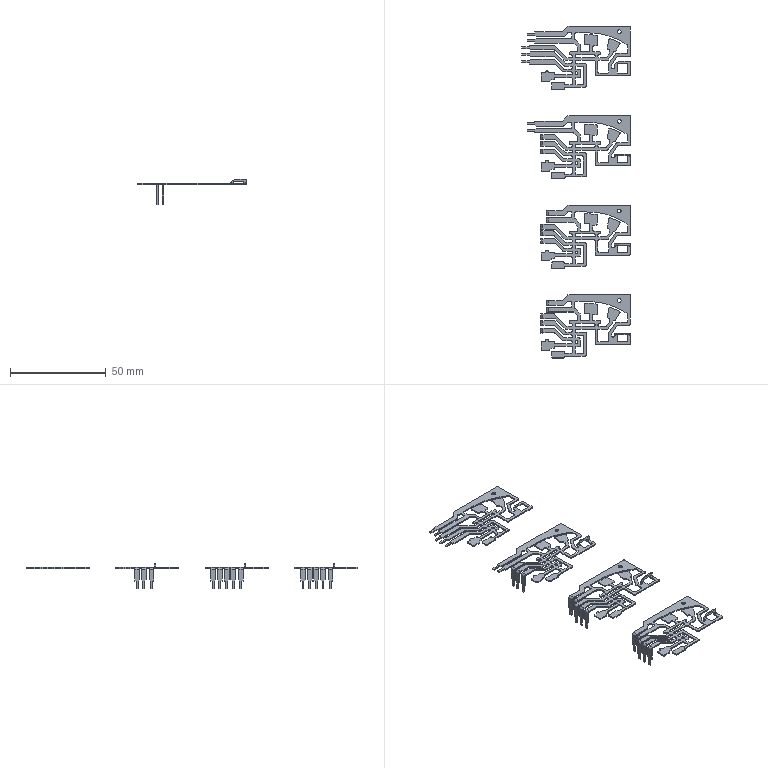Part | NX | features BREP 4 | 4 solids | 1138 faces | box 57.003 x 173.8 x 13.3 mm | volume 1971 mm3 | plane 616 | cylinder 522 | commonest cylinder face diameters 1 x479 2.2 x19 2 x4 69.173 x4 72.496 x4 72.701 x4